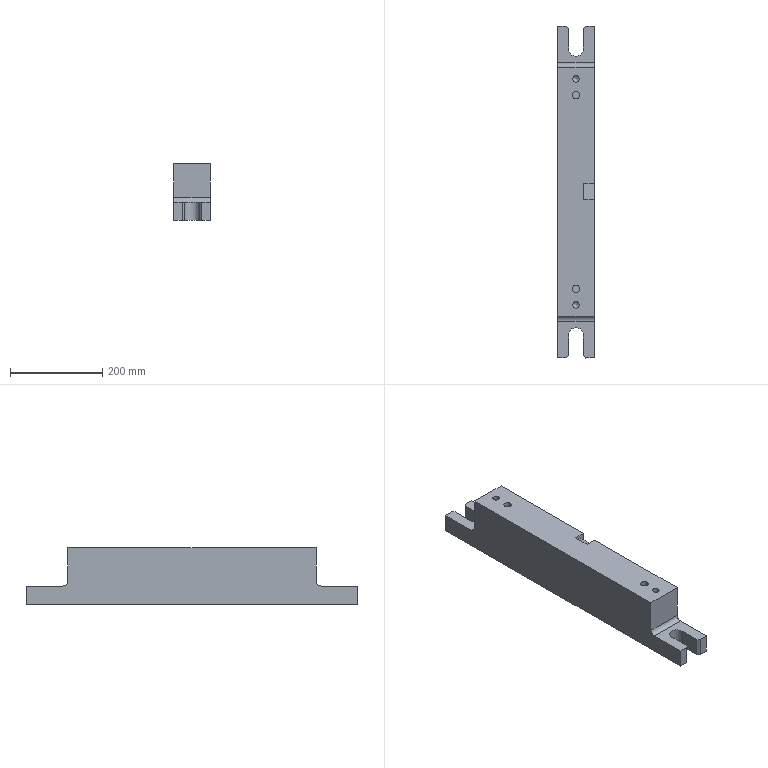Part | NX | features LIN_SOLID_COLOR 2 | 1 solid | 35 faces | box 80 x 720 x 123.5 mm | volume 5716892 mm3 | plane 25 | cylinder 8 | cone 2 | commonest cylinder face diameters 14 x2 16.002 x2 20 x2 32 x2
STEP:
#1=CARTESIAN_POINT('',(-314.,270.,-180.));
#2=VERTEX_POINT('',#1);
#3=CARTESIAN_POINT('',(-234.,270.,-180.));
#4=VERTEX_POINT('',#3);
#5=CARTESIAN_POINT('',(-234.,270.,-180.));
#6=DIRECTION('',(-1.,0.,0.));
#7=VECTOR('',#6,1000.);
#8=LINE('',#5,#7);
#9=EDGE_CURVE('',#2,#4,#8,.F.);
#10=ORIENTED_EDGE('',*,*,#9,.F.);
#11=CARTESIAN_POINT('',(-314.,270.,-106.5));
#12=VERTEX_POINT('',#11);
#13=CARTESIAN_POINT('',(-314.,270.,-101.5));
#14=DIRECTION('',(0.,0.,1.));
#15=VECTOR('',#14,1000.);
#16=LINE('',#13,#15);
#17=EDGE_CURVE('',#2,#12,#16,.T.);
#18=ORIENTED_EDGE('',*,*,#17,.T.);
#19=CARTESIAN_POINT('',(-234.,270.,-106.5));
#20=VERTEX_POINT('',#19);
#21=CARTESIAN_POINT('',(-254.,270.,-106.5));
#22=DIRECTION('',(1.,0.,0.));
#23=VECTOR('',#22,1000.);
#24=LINE('',#21,#23);
#25=EDGE_CURVE('',#12,#20,#24,.T.);
#26=ORIENTED_EDGE('',*,*,#25,.T.);
#27=CARTESIAN_POINT('',(-234.,270.,-101.5));
#28=DIRECTION('',(0.,0.,1.));
#29=VECTOR('',#28,1000.);
#30=LINE('',#27,#29);
#31=EDGE_CURVE('',#4,#20,#30,.T.);
#32=ORIENTED_EDGE('',*,*,#31,.F.);
#33=EDGE_LOOP('',(#10,#18,#26,#32));
#34=FACE_BOUND('',#33,.T.);
#35=CARTESIAN_POINT('',(-254.,270.,-101.5));
#36=DIRECTION('',(0.,-1.,0.));
#37=DIRECTION('',(0.,0.,1.));
#38=AXIS2_PLACEMENT_3D('',#35,#36,#37);
#39=PLANE('',#38);
#40=ADVANCED_FACE('',(#34),#39,.F.);
#41=CARTESIAN_POINT('',(-234.,360.,-230.));
#42=VERTEX_POINT('',#41);
#43=CARTESIAN_POINT('',(-234.,-360.,-230.));
#44=VERTEX_POINT('',#43);
#45=CARTESIAN_POINT('',(-234.,0.,-230.));
#46=DIRECTION('',(0.,-1.,0.));
#47=VECTOR('',#46,1000.);
#48=LINE('',#45,#47);
#49=EDGE_CURVE('',#42,#44,#48,.T.);
#50=ORIENTED_EDGE('',*,*,#49,.T.);
#51=CARTESIAN_POINT('',(-253.,-360.,-230.));
#52=VERTEX_POINT('',#51);
#53=CARTESIAN_POINT('',(436.,-360.,-230.));
#54=DIRECTION('',(1.,0.,0.));
#55=VECTOR('',#54,1000.);
#56=LINE('',#53,#55);
#57=EDGE_CURVE('',#52,#44,#56,.T.);
#58=ORIENTED_EDGE('',*,*,#57,.F.);
#59=CARTESIAN_POINT('',(-258.,-355.,-230.));
#60=VERTEX_POINT('',#59);
#61=CARTESIAN_POINT('',(-126144.583,125531.583,-230.));
#62=DIRECTION('',(-0.7071,0.7071,0.));
#63=VECTOR('',#62,1000.);
#64=LINE('',#61,#63);
#65=EDGE_CURVE('',#52,#60,#64,.T.);
#66=ORIENTED_EDGE('',*,*,#65,.T.);
#67=CARTESIAN_POINT('',(-258.,-310.,-230.));
#68=VERTEX_POINT('',#67);
#69=CARTESIAN_POINT('',(-258.,-1858.277,-230.));
#70=DIRECTION('',(0.,-1.,0.));
#71=VECTOR('',#70,1000.);
#72=LINE('',#69,#71);
#73=EDGE_CURVE('',#68,#60,#72,.T.);
#74=ORIENTED_EDGE('',*,*,#73,.F.);
#75=CARTESIAN_POINT('',(-290.,-310.,-230.));
#76=VERTEX_POINT('',#75);
#77=CARTESIAN_POINT('',(-274.,-310.,-230.));
#78=DIRECTION('',(0.,0.,-1.));
#79=DIRECTION('',(-1.,0.,0.));
#80=AXIS2_PLACEMENT_3D('',#77,#78,#79);
#81=CIRCLE('',#80,16.);
#82=EDGE_CURVE('',#76,#68,#81,.T.);
#83=ORIENTED_EDGE('',*,*,#82,.F.);
#84=CARTESIAN_POINT('',(-290.,-355.,-230.));
#85=VERTEX_POINT('',#84);
#86=CARTESIAN_POINT('',(-290.,-1858.277,-230.));
#87=DIRECTION('',(0.,1.,0.));
#88=VECTOR('',#87,1000.);
#89=LINE('',#86,#88);
#90=EDGE_CURVE('',#85,#76,#89,.T.);
#91=ORIENTED_EDGE('',*,*,#90,.F.);
#92=CARTESIAN_POINT('',(-295.,-360.,-230.));
#93=VERTEX_POINT('',#92);
#94=CARTESIAN_POINT('',(-127663.859,-127728.859,-230.));
#95=DIRECTION('',(-0.7071,-0.7071,0.));
#96=VECTOR('',#95,1000.);
#97=LINE('',#94,#96);
#98=EDGE_CURVE('',#85,#93,#97,.T.);
#99=ORIENTED_EDGE('',*,*,#98,.T.);
#100=CARTESIAN_POINT('',(-314.,-360.,-230.));
#101=VERTEX_POINT('',#100);
#102=CARTESIAN_POINT('',(436.,-360.,-230.));
#103=DIRECTION('',(1.,0.,0.));
#104=VECTOR('',#103,1000.);
#105=LINE('',#102,#104);
#106=EDGE_CURVE('',#101,#93,#105,.T.);
#107=ORIENTED_EDGE('',*,*,#106,.F.);
#108=CARTESIAN_POINT('',(-314.,360.,-230.));
#109=VERTEX_POINT('',#108);
#110=CARTESIAN_POINT('',(-314.,0.,-230.));
#111=DIRECTION('',(0.,-1.,0.));
#112=VECTOR('',#111,1000.);
#113=LINE('',#110,#112);
#114=EDGE_CURVE('',#109,#101,#113,.T.);
#115=ORIENTED_EDGE('',*,*,#114,.F.);
#116=CARTESIAN_POINT('',(-295.,360.,-230.));
#117=VERTEX_POINT('',#116);
#118=CARTESIAN_POINT('',(436.,360.,-230.));
#119=DIRECTION('',(1.,0.,0.));
#120=VECTOR('',#119,1000.);
#121=LINE('',#118,#120);
#122=EDGE_CURVE('',#109,#117,#121,.T.);
#123=ORIENTED_EDGE('',*,*,#122,.T.);
#124=CARTESIAN_POINT('',(-290.,355.,-230.));
#125=VERTEX_POINT('',#124);
#126=CARTESIAN_POINT('',(-127663.859,127728.859,-230.));
#127=DIRECTION('',(-0.7071,0.7071,0.));
#128=VECTOR('',#127,1000.);
#129=LINE('',#126,#128);
#130=EDGE_CURVE('',#125,#117,#129,.T.);
#131=ORIENTED_EDGE('',*,*,#130,.F.);
#132=CARTESIAN_POINT('',(-290.,310.,-230.));
#133=VERTEX_POINT('',#132);
#134=CARTESIAN_POINT('',(-290.,1858.277,-230.));
#135=DIRECTION('',(0.,-1.,0.));
#136=VECTOR('',#135,1000.);
#137=LINE('',#134,#136);
#138=EDGE_CURVE('',#125,#133,#137,.T.);
#139=ORIENTED_EDGE('',*,*,#138,.T.);
#140=CARTESIAN_POINT('',(-258.,310.,-230.));
#141=VERTEX_POINT('',#140);
#142=CARTESIAN_POINT('',(-274.,310.,-230.));
#143=DIRECTION('',(0.,0.,1.));
#144=DIRECTION('',(-1.,0.,0.));
#145=AXIS2_PLACEMENT_3D('',#142,#143,#144);
#146=CIRCLE('',#145,16.);
#147=EDGE_CURVE('',#133,#141,#146,.T.);
#148=ORIENTED_EDGE('',*,*,#147,.T.);
#149=CARTESIAN_POINT('',(-258.,355.,-230.));
#150=VERTEX_POINT('',#149);
#151=CARTESIAN_POINT('',(-258.,1858.277,-230.));
#152=DIRECTION('',(0.,1.,0.));
#153=VECTOR('',#152,1000.);
#154=LINE('',#151,#153);
#155=EDGE_CURVE('',#141,#150,#154,.T.);
#156=ORIENTED_EDGE('',*,*,#155,.T.);
#157=CARTESIAN_POINT('',(-253.,360.,-230.));
#158=VERTEX_POINT('',#157);
#159=CARTESIAN_POINT('',(-126144.583,-125531.583,-230.));
#160=DIRECTION('',(-0.7071,-0.7071,0.));
#161=VECTOR('',#160,1000.);
#162=LINE('',#159,#161);
#163=EDGE_CURVE('',#158,#150,#162,.T.);
#164=ORIENTED_EDGE('',*,*,#163,.F.);
#165=CARTESIAN_POINT('',(436.,360.,-230.));
#166=DIRECTION('',(1.,0.,0.));
#167=VECTOR('',#166,1000.);
#168=LINE('',#165,#167);
#169=EDGE_CURVE('',#158,#42,#168,.T.);
#170=ORIENTED_EDGE('',*,*,#169,.T.);
#171=EDGE_LOOP('',(#50,#58,#66,#74,#83,#91,#99,#107,#115,#123,#131,#139,#148,#156,#164,#170));
#172=FACE_BOUND('',#171,.T.);
#173=CARTESIAN_POINT('',(-114.,0.,-230.));
#174=DIRECTION('',(0.,0.,1.));
#175=DIRECTION('',(1.,0.,0.));
#176=AXIS2_PLACEMENT_3D('',#173,#174,#175);
#177=PLANE('',#176);
#178=ADVANCED_FACE('',(#172),#177,.F.);
#179=CARTESIAN_POINT('',(-234.,-270.,-106.5));
#180=VERTEX_POINT('',#179);
#181=CARTESIAN_POINT('',(-234.,-17.5,-106.5));
#182=VERTEX_POINT('',#181);
#183=CARTESIAN_POINT('',(-234.,0.,-106.5));
#184=DIRECTION('',(0.,1.,0.));
#185=VECTOR('',#184,1000.);
#186=LINE('',#183,#185);
#187=EDGE_CURVE('',#180,#182,#186,.T.);
#188=ORIENTED_EDGE('',*,*,#187,.T.);
#189=CARTESIAN_POINT('',(-257.475,-17.5,-106.5));
#190=VERTEX_POINT('',#189);
#191=CARTESIAN_POINT('',(476.,-17.5,-106.5));
#192=DIRECTION('',(-1.,0.,0.));
#193=VECTOR('',#192,1000.);
#194=LINE('',#191,#193);
#195=EDGE_CURVE('',#182,#190,#194,.T.);
#196=ORIENTED_EDGE('',*,*,#195,.T.);
#197=CARTESIAN_POINT('',(-257.475,17.5,-106.5));
#198=VERTEX_POINT('',#197);
#199=CARTESIAN_POINT('',(-257.475,0.,-106.5));
#200=DIRECTION('',(0.,1.,0.));
#201=VECTOR('',#200,1000.);
#202=LINE('',#199,#201);
#203=EDGE_CURVE('',#198,#190,#202,.F.);
#204=ORIENTED_EDGE('',*,*,#203,.F.);
#205=CARTESIAN_POINT('',(-234.,17.5,-106.5));
#206=VERTEX_POINT('',#205);
#207=CARTESIAN_POINT('',(476.,17.5,-106.5));
#208=DIRECTION('',(1.,0.,0.));
#209=VECTOR('',#208,1000.);
#210=LINE('',#207,#209);
#211=EDGE_CURVE('',#198,#206,#210,.T.);
#212=ORIENTED_EDGE('',*,*,#211,.T.);
#213=CARTESIAN_POINT('',(-234.,0.,-106.5));
#214=DIRECTION('',(0.,1.,0.));
#215=VECTOR('',#214,1000.);
#216=LINE('',#213,#215);
#217=EDGE_CURVE('',#206,#20,#216,.T.);
#218=ORIENTED_EDGE('',*,*,#217,.T.);
#219=ORIENTED_EDGE('',*,*,#25,.F.);
#220=CARTESIAN_POINT('',(-314.,-270.,-106.5));
#221=VERTEX_POINT('',#220);
#222=CARTESIAN_POINT('',(-314.,0.,-106.5));
#223=DIRECTION('',(0.,1.,0.));
#224=VECTOR('',#223,1000.);
#225=LINE('',#222,#224);
#226=EDGE_CURVE('',#221,#12,#225,.T.);
#227=ORIENTED_EDGE('',*,*,#226,.F.);
#228=CARTESIAN_POINT('',(476.,-270.,-106.5));
#229=DIRECTION('',(-1.,0.,0.));
#230=VECTOR('',#229,1000.);
#231=LINE('',#228,#230);
#232=EDGE_CURVE('',#180,#221,#231,.T.);
#233=ORIENTED_EDGE('',*,*,#232,.F.);
#234=EDGE_LOOP('',(#188,#196,#204,#212,#218,#219,#227,#233));
#235=FACE_BOUND('',#234,.T.);
#236=CARTESIAN_POINT('',(-282.001,-210.,-106.5));
#237=VERTEX_POINT('',#236);
#238=CARTESIAN_POINT('',(-274.,-210.,-106.5));
#239=DIRECTION('',(0.,0.,-1.));
#240=DIRECTION('',(-1.,0.,0.));
#241=AXIS2_PLACEMENT_3D('',#238,#239,#240);
#242=CIRCLE('',#241,8.001);
#243=EDGE_CURVE('',#237,#237,#242,.F.);
#244=ORIENTED_EDGE('',*,*,#243,.F.);
#245=EDGE_LOOP('',(#244));
#246=FACE_BOUND('',#245,.T.);
#247=CARTESIAN_POINT('',(-281.,-245.,-106.5));
#248=VERTEX_POINT('',#247);
#249=CARTESIAN_POINT('',(-274.,-245.,-106.5));
#250=DIRECTION('',(0.,0.,-1.));
#251=DIRECTION('',(-1.,0.,0.));
#252=AXIS2_PLACEMENT_3D('',#249,#250,#251);
#253=CIRCLE('',#252,7.);
#254=EDGE_CURVE('',#248,#248,#253,.T.);
#255=ORIENTED_EDGE('',*,*,#254,.T.);
#256=EDGE_LOOP('',(#255));
#257=FACE_BOUND('',#256,.T.);
#258=CARTESIAN_POINT('',(-281.,245.,-106.5));
#259=VERTEX_POINT('',#258);
#260=CARTESIAN_POINT('',(-274.,245.,-106.5));
#261=DIRECTION('',(0.,0.,-1.));
#262=DIRECTION('',(-1.,0.,0.));
#263=AXIS2_PLACEMENT_3D('',#260,#261,#262);
#264=CIRCLE('',#263,7.);
#265=EDGE_CURVE('',#259,#259,#264,.T.);
#266=ORIENTED_EDGE('',*,*,#265,.T.);
#267=EDGE_LOOP('',(#266));
#268=FACE_BOUND('',#267,.T.);
#269=CARTESIAN_POINT('',(-282.001,210.,-106.5));
#270=VERTEX_POINT('',#269);
#271=CARTESIAN_POINT('',(-274.,210.,-106.5));
#272=DIRECTION('',(0.,0.,-1.));
#273=DIRECTION('',(-1.,0.,0.));
#274=AXIS2_PLACEMENT_3D('',#271,#272,#273);
#275=CIRCLE('',#274,8.001);
#276=EDGE_CURVE('',#270,#270,#275,.T.);
#277=ORIENTED_EDGE('',*,*,#276,.T.);
#278=EDGE_LOOP('',(#277));
#279=FACE_BOUND('',#278,.T.);
#280=CARTESIAN_POINT('',(476.,0.,-106.5));
#281=DIRECTION('',(0.,0.,-1.));
#282=DIRECTION('',(-1.,0.,0.));
#283=AXIS2_PLACEMENT_3D('',#280,#281,#282);
#284=PLANE('',#283);
#285=ADVANCED_FACE('',(#235,#246,#257,#268,#279),#284,.F.);
#286=CARTESIAN_POINT('',(-234.,17.5,-122.937));
#287=VERTEX_POINT('',#286);
#288=CARTESIAN_POINT('',(-234.,17.5,-101.5));
#289=DIRECTION('',(0.,0.,-1.));
#290=VECTOR('',#289,1000.);
#291=LINE('',#288,#290);
#292=EDGE_CURVE('',#206,#287,#291,.T.);
#293=ORIENTED_EDGE('',*,*,#292,.T.);
#294=CARTESIAN_POINT('',(-234.,-17.5,-122.937));
#295=VERTEX_POINT('',#294);
#296=CARTESIAN_POINT('',(-234.,0.,-122.937));
#297=DIRECTION('',(0.,-1.,0.));
#298=VECTOR('',#297,1000.);
#299=LINE('',#296,#298);
#300=EDGE_CURVE('',#295,#287,#299,.F.);
#301=ORIENTED_EDGE('',*,*,#300,.F.);
#302=CARTESIAN_POINT('',(-234.,-17.5,-101.5));
#303=DIRECTION('',(0.,0.,1.));
#304=VECTOR('',#303,1000.);
#305=LINE('',#302,#304);
#306=EDGE_CURVE('',#295,#182,#305,.T.);
#307=ORIENTED_EDGE('',*,*,#306,.T.);
#308=ORIENTED_EDGE('',*,*,#187,.F.);
#309=CARTESIAN_POINT('',(-234.,-270.,-180.));
#310=VERTEX_POINT('',#309);
#311=CARTESIAN_POINT('',(-234.,-270.,-101.5));
#312=DIRECTION('',(0.,0.,1.));
#313=VECTOR('',#312,1000.);
#314=LINE('',#311,#313);
#315=EDGE_CURVE('',#310,#180,#314,.T.);
#316=ORIENTED_EDGE('',*,*,#315,.F.);
#317=CARTESIAN_POINT('',(-234.,-280.,-190.));
#318=VERTEX_POINT('',#317);
#319=CARTESIAN_POINT('',(-234.,-280.,-180.));
#320=DIRECTION('',(-1.,0.,0.));
#321=DIRECTION('',(0.,0.,1.));
#322=AXIS2_PLACEMENT_3D('',#319,#320,#321);
#323=CIRCLE('',#322,10.);
#324=EDGE_CURVE('',#310,#318,#323,.T.);
#325=ORIENTED_EDGE('',*,*,#324,.T.);
#326=CARTESIAN_POINT('',(-234.,-360.,-190.));
#327=VERTEX_POINT('',#326);
#328=CARTESIAN_POINT('',(-234.,-320.,-190.));
#329=DIRECTION('',(0.,-1.,0.));
#330=VECTOR('',#329,1000.);
#331=LINE('',#328,#330);
#332=EDGE_CURVE('',#318,#327,#331,.T.);
#333=ORIENTED_EDGE('',*,*,#332,.T.);
#334=CARTESIAN_POINT('',(-234.,-360.,-131.5));
#335=DIRECTION('',(0.,0.,1.));
#336=VECTOR('',#335,1000.);
#337=LINE('',#334,#336);
#338=EDGE_CURVE('',#44,#327,#337,.T.);
#339=ORIENTED_EDGE('',*,*,#338,.F.);
#340=ORIENTED_EDGE('',*,*,#49,.F.);
#341=CARTESIAN_POINT('',(-234.,360.,-190.));
#342=VERTEX_POINT('',#341);
#343=CARTESIAN_POINT('',(-234.,360.,-131.5));
#344=DIRECTION('',(0.,0.,1.));
#345=VECTOR('',#344,1000.);
#346=LINE('',#343,#345);
#347=EDGE_CURVE('',#42,#342,#346,.T.);
#348=ORIENTED_EDGE('',*,*,#347,.T.);
#349=CARTESIAN_POINT('',(-234.,280.,-190.));
#350=VERTEX_POINT('',#349);
#351=CARTESIAN_POINT('',(-234.,320.,-190.));
#352=DIRECTION('',(0.,1.,0.));
#353=VECTOR('',#352,1000.);
#354=LINE('',#351,#353);
#355=EDGE_CURVE('',#350,#342,#354,.T.);
#356=ORIENTED_EDGE('',*,*,#355,.F.);
#357=CARTESIAN_POINT('',(-234.,280.,-180.));
#358=DIRECTION('',(1.,0.,0.));
#359=DIRECTION('',(0.,0.,1.));
#360=AXIS2_PLACEMENT_3D('',#357,#358,#359);
#361=CIRCLE('',#360,10.);
#362=EDGE_CURVE('',#4,#350,#361,.T.);
#363=ORIENTED_EDGE('',*,*,#362,.F.);
#364=ORIENTED_EDGE('',*,*,#31,.T.);
#365=ORIENTED_EDGE('',*,*,#217,.F.);
#366=EDGE_LOOP('',(#293,#301,#307,#308,#316,#325,#333,#339,#340,#348,#356,#363,#364,#365));
#367=FACE_BOUND('',#366,.T.);
#368=CARTESIAN_POINT('',(-234.,0.,-101.5));
#369=DIRECTION('',(-1.,0.,0.));
#370=DIRECTION('',(0.,0.,1.));
#371=AXIS2_PLACEMENT_3D('',#368,#369,#370);
#372=PLANE('',#371);
#373=ADVANCED_FACE('',(#367),#372,.F.);
#374=ORIENTED_EDGE('',*,*,#114,.T.);
#375=CARTESIAN_POINT('',(-314.,-360.,-190.));
#376=VERTEX_POINT('',#375);
#377=CARTESIAN_POINT('',(-314.,-360.,-111.5));
#378=DIRECTION('',(0.,0.,1.));
#379=VECTOR('',#378,1000.);
#380=LINE('',#377,#379);
#381=EDGE_CURVE('',#101,#376,#380,.T.);
#382=ORIENTED_EDGE('',*,*,#381,.T.);
#383=CARTESIAN_POINT('',(-314.,-280.,-190.));
#384=VERTEX_POINT('',#383);
#385=CARTESIAN_POINT('',(-314.,-10.,-190.));
#386=DIRECTION('',(0.,1.,0.));
#387=VECTOR('',#386,1000.);
#388=LINE('',#385,#387);
#389=EDGE_CURVE('',#376,#384,#388,.T.);
#390=ORIENTED_EDGE('',*,*,#389,.T.);
#391=CARTESIAN_POINT('',(-314.,-270.,-180.));
#392=VERTEX_POINT('',#391);
#393=CARTESIAN_POINT('',(-314.,-280.,-180.));
#394=DIRECTION('',(-1.,0.,0.));
#395=DIRECTION('',(0.,0.,1.));
#396=AXIS2_PLACEMENT_3D('',#393,#394,#395);
#397=CIRCLE('',#396,10.);
#398=EDGE_CURVE('',#384,#392,#397,.F.);
#399=ORIENTED_EDGE('',*,*,#398,.T.);
#400=CARTESIAN_POINT('',(-314.,-270.,-101.5));
#401=DIRECTION('',(0.,0.,1.));
#402=VECTOR('',#401,1000.);
#403=LINE('',#400,#402);
#404=EDGE_CURVE('',#221,#392,#403,.F.);
#405=ORIENTED_EDGE('',*,*,#404,.F.);
#406=ORIENTED_EDGE('',*,*,#226,.T.);
#407=ORIENTED_EDGE('',*,*,#17,.F.);
#408=CARTESIAN_POINT('',(-314.,280.,-190.));
#409=VERTEX_POINT('',#408);
#410=CARTESIAN_POINT('',(-314.,280.,-180.));
#411=DIRECTION('',(1.,0.,0.));
#412=DIRECTION('',(0.,0.,1.));
#413=AXIS2_PLACEMENT_3D('',#410,#411,#412);
#414=CIRCLE('',#413,10.);
#415=EDGE_CURVE('',#409,#2,#414,.F.);
#416=ORIENTED_EDGE('',*,*,#415,.F.);
#417=CARTESIAN_POINT('',(-314.,360.,-190.));
#418=VERTEX_POINT('',#417);
#419=CARTESIAN_POINT('',(-314.,10.,-190.));
#420=DIRECTION('',(0.,-1.,0.));
#421=VECTOR('',#420,1000.);
#422=LINE('',#419,#421);
#423=EDGE_CURVE('',#418,#409,#422,.T.);
#424=ORIENTED_EDGE('',*,*,#423,.F.);
#425=CARTESIAN_POINT('',(-314.,360.,-111.5));
#426=DIRECTION('',(0.,0.,1.));
#427=VECTOR('',#426,1000.);
#428=LINE('',#425,#427);
#429=EDGE_CURVE('',#109,#418,#428,.T.);
#430=ORIENTED_EDGE('',*,*,#429,.F.);
#431=EDGE_LOOP('',(#374,#382,#390,#399,#405,#406,#407,#416,#424,#430));
#432=FACE_BOUND('',#431,.T.);
#433=CARTESIAN_POINT('',(-314.,0.,-101.5));
#434=DIRECTION('',(-1.,0.,0.));
#435=DIRECTION('',(0.,0.,1.));
#436=AXIS2_PLACEMENT_3D('',#433,#434,#435);
#437=PLANE('',#436);
#438=ADVANCED_FACE('',(#432),#437,.T.);
#439=CARTESIAN_POINT('',(-267.,-245.,-146.5));
#440=VERTEX_POINT('',#439);
#441=CARTESIAN_POINT('',(-274.,-245.,-146.5));
#442=DIRECTION('',(0.,0.,1.));
#443=DIRECTION('',(1.,0.,0.));
#444=AXIS2_PLACEMENT_3D('',#441,#442,#443);
#445=CIRCLE('',#444,7.);
#446=EDGE_CURVE('',#440,#440,#445,.T.);
#447=ORIENTED_EDGE('',*,*,#446,.F.);
#448=EDGE_LOOP('',(#447));
#449=FACE_BOUND('',#448,.T.);
#450=ORIENTED_EDGE('',*,*,#254,.F.);
#451=EDGE_LOOP('',(#450));
#452=FACE_BOUND('',#451,.T.);
#453=CARTESIAN_POINT('',(-274.,-245.,-106.4));
#454=DIRECTION('',(0.,0.,-1.));
#455=DIRECTION('',(1.,0.,0.));
#456=AXIS2_PLACEMENT_3D('',#453,#454,#455);
#457=CYLINDRICAL_SURFACE('',#456,7.);
#458=ADVANCED_FACE('',(#449,#452),#457,.F.);
#459=ORIENTED_EDGE('',*,*,#446,.T.);
#460=EDGE_LOOP('',(#459));
#461=FACE_BOUND('',#460,.T.);
#462=CARTESIAN_POINT('',(-274.,-245.,-150.541));
#463=VERTEX_POINT('',#462);
#464=VERTEX_LOOP('',#463);
#465=FACE_BOUND('',#464,.T.);
#466=CARTESIAN_POINT('',(-274.,-245.,-150.541));
#467=DIRECTION('',(0.,0.,1.));
#468=DIRECTION('',(1.,0.,0.));
#469=AXIS2_PLACEMENT_3D('',#466,#467,#468);
#470=CONICAL_SURFACE('',#469,0.,1.047);
#471=ADVANCED_FACE('',(#461,#465),#470,.F.);
#472=CARTESIAN_POINT('',(-267.,245.,-146.5));
#473=VERTEX_POINT('',#472);
#474=CARTESIAN_POINT('',(-274.,245.,-146.5));
#475=DIRECTION('',(0.,0.,1.));
#476=DIRECTION('',(1.,0.,0.));
#477=AXIS2_PLACEMENT_3D('',#474,#475,#476);
#478=CIRCLE('',#477,7.);
#479=EDGE_CURVE('',#473,#473,#478,.T.);
#480=ORIENTED_EDGE('',*,*,#479,.F.);
#481=EDGE_LOOP('',(#480));
#482=FACE_BOUND('',#481,.T.);
#483=ORIENTED_EDGE('',*,*,#265,.F.);
#484=EDGE_LOOP('',(#483));
#485=FACE_BOUND('',#484,.T.);
#486=CARTESIAN_POINT('',(-274.,245.,-106.4));
#487=DIRECTION('',(0.,0.,-1.));
#488=DIRECTION('',(1.,0.,0.));
#489=AXIS2_PLACEMENT_3D('',#486,#487,#488);
#490=CYLINDRICAL_SURFACE('',#489,7.);
#491=ADVANCED_FACE('',(#482,#485),#490,.F.);
#492=ORIENTED_EDGE('',*,*,#479,.T.);
#493=EDGE_LOOP('',(#492));
#494=FACE_BOUND('',#493,.T.);
#495=CARTESIAN_POINT('',(-274.,245.,-150.541));
#496=VERTEX_POINT('',#495);
#497=VERTEX_LOOP('',#496);
#498=FACE_BOUND('',#497,.T.);
#499=CARTESIAN_POINT('',(-274.,245.,-150.541));
#500=DIRECTION('',(0.,0.,1.));
#501=DIRECTION('',(1.,0.,0.));
#502=AXIS2_PLACEMENT_3D('',#499,#500,#501);
#503=CONICAL_SURFACE('',#502,0.,1.047);
#504=ADVANCED_FACE('',(#494,#498),#503,.F.);
#505=CARTESIAN_POINT('',(-265.999,210.,-146.5));
#506=VERTEX_POINT('',#505);
#507=CARTESIAN_POINT('',(-274.,210.,-146.5));
#508=DIRECTION('',(0.,0.,1.));
#509=DIRECTION('',(1.,0.,0.));
#510=AXIS2_PLACEMENT_3D('',#507,#508,#509);
#511=CIRCLE('',#510,8.001);
#512=EDGE_CURVE('',#506,#506,#511,.T.);
#513=ORIENTED_EDGE('',*,*,#512,.F.);
#514=EDGE_LOOP('',(#513));
#515=FACE_BOUND('',#514,.T.);
#516=ORIENTED_EDGE('',*,*,#276,.F.);
#517=EDGE_LOOP('',(#516));
#518=FACE_BOUND('',#517,.T.);
#519=CARTESIAN_POINT('',(-274.,210.,-339.5));
#520=DIRECTION('',(0.,0.,1.));
#521=DIRECTION('',(1.,0.,0.));
#522=AXIS2_PLACEMENT_3D('',#519,#520,#521);
#523=CYLINDRICAL_SURFACE('',#522,8.001);
#524=ADVANCED_FACE('',(#515,#518),#523,.F.);
#525=ORIENTED_EDGE('',*,*,#243,.T.);
#526=EDGE_LOOP('',(#525));
#527=FACE_BOUND('',#526,.T.);
#528=CARTESIAN_POINT('',(-265.999,-210.,-146.5));
#529=VERTEX_POINT('',#528);
#530=CARTESIAN_POINT('',(-274.,-210.,-146.5));
#531=DIRECTION('',(0.,0.,1.));
#532=DIRECTION('',(1.,0.,0.));
#533=AXIS2_PLACEMENT_3D('',#530,#531,#532);
#534=CIRCLE('',#533,8.001);
#535=EDGE_CURVE('',#529,#529,#534,.F.);
#536=ORIENTED_EDGE('',*,*,#535,.T.);
#537=EDGE_LOOP('',(#536));
#538=FACE_BOUND('',#537,.T.);
#539=CARTESIAN_POINT('',(-274.,-210.,-304.5));
#540=DIRECTION('',(0.,0.,1.));
#541=DIRECTION('',(1.,0.,0.));
#542=AXIS2_PLACEMENT_3D('',#539,#540,#541);
#543=CYLINDRICAL_SURFACE('',#542,8.001);
#544=ADVANCED_FACE('',(#527,#538),#543,.F.);
#545=ORIENTED_EDGE('',*,*,#404,.T.);
#546=CARTESIAN_POINT('',(-234.,-270.,-180.));
#547=DIRECTION('',(-1.,0.,0.));
#548=VECTOR('',#547,1000.);
#549=LINE('',#546,#548);
#550=EDGE_CURVE('',#392,#310,#549,.F.);
#551=ORIENTED_EDGE('',*,*,#550,.T.);
#552=ORIENTED_EDGE('',*,*,#315,.T.);
#553=ORIENTED_EDGE('',*,*,#232,.T.);
#554=EDGE_LOOP('',(#545,#551,#552,#553));
#555=FACE_BOUND('',#554,.T.);
#556=CARTESIAN_POINT('',(271.,-270.,-71.5));
#557=DIRECTION('',(0.,-1.,0.));
#558=DIRECTION('',(0.,0.,-1.));
#559=AXIS2_PLACEMENT_3D('',#556,#557,#558);
#560=PLANE('',#559);
#561=ADVANCED_FACE('',(#555),#560,.T.);
#562=ORIENTED_EDGE('',*,*,#106,.T.);
#563=CARTESIAN_POINT('',(-295.,-360.,-190.));
#564=VERTEX_POINT('',#563);
#565=CARTESIAN_POINT('',(-295.,-360.,-200.));
#566=DIRECTION('',(0.,0.,1.));
#567=VECTOR('',#566,1000.);
#568=LINE('',#565,#567);
#569=EDGE_CURVE('',#93,#564,#568,.T.);
#570=ORIENTED_EDGE('',*,*,#569,.T.);
#571=CARTESIAN_POINT('',(436.,-360.,-190.));
#572=DIRECTION('',(-1.,0.,0.));
#573=VECTOR('',#572,1000.);
#574=LINE('',#571,#573);
#575=EDGE_CURVE('',#564,#376,#574,.T.);
#576=ORIENTED_EDGE('',*,*,#575,.T.);
#577=ORIENTED_EDGE('',*,*,#381,.F.);
#578=EDGE_LOOP('',(#562,#570,#576,#577));
#579=FACE_BOUND('',#578,.T.);
#580=CARTESIAN_POINT('',(436.,-360.,-131.5));
#581=DIRECTION('',(0.,-1.,0.));
#582=DIRECTION('',(0.,0.,-1.));
#583=AXIS2_PLACEMENT_3D('',#580,#581,#582);
#584=PLANE('',#583);
#585=ADVANCED_FACE('',(#579),#584,.T.);
#586=ORIENTED_EDGE('',*,*,#98,.F.);
#587=CARTESIAN_POINT('',(-290.,-355.,-190.));
#588=VERTEX_POINT('',#587);
#589=CARTESIAN_POINT('',(-290.,-355.,-230.));
#590=DIRECTION('',(0.,0.,-1.));
#591=VECTOR('',#590,1000.);
#592=LINE('',#589,#591);
#593=EDGE_CURVE('',#588,#85,#592,.T.);
#594=ORIENTED_EDGE('',*,*,#593,.F.);
#595=CARTESIAN_POINT('',(-64.5,-129.5,-190.));
#596=DIRECTION('',(0.7071,0.7071,0.));
#597=VECTOR('',#596,1000.);
#598=LINE('',#595,#597);
#599=EDGE_CURVE('',#564,#588,#598,.T.);
#600=ORIENTED_EDGE('',*,*,#599,.F.);
#601=ORIENTED_EDGE('',*,*,#569,.F.);
#602=EDGE_LOOP('',(#586,#594,#600,#601));
#603=FACE_BOUND('',#602,.T.);
#604=CARTESIAN_POINT('',(-295.,-360.,-131.5));
#605=DIRECTION('',(0.7071,-0.7071,0.));
#606=DIRECTION('',(0.,0.,-1.));
#607=AXIS2_PLACEMENT_3D('',#604,#605,#606);
#608=PLANE('',#607);
#609=ADVANCED_FACE('',(#603),#608,.T.);
#610=CARTESIAN_POINT('',(-290.,-310.,-190.));
#611=VERTEX_POINT('',#610);
#612=CARTESIAN_POINT('',(-290.,-30.,-190.));
#613=DIRECTION('',(0.,-1.,0.));
#614=VECTOR('',#613,1000.);
#615=LINE('',#612,#614);
#616=EDGE_CURVE('',#611,#588,#615,.T.);
#617=ORIENTED_EDGE('',*,*,#616,.T.);
#618=ORIENTED_EDGE('',*,*,#593,.T.);
#619=ORIENTED_EDGE('',*,*,#90,.T.);
#620=CARTESIAN_POINT('',(-290.,-310.,-305.));
#621=DIRECTION('',(0.,0.,1.));
#622=VECTOR('',#621,1000.);
#623=LINE('',#620,#622);
#624=EDGE_CURVE('',#611,#76,#623,.F.);
#625=ORIENTED_EDGE('',*,*,#624,.F.);
#626=EDGE_LOOP('',(#617,#618,#619,#625));
#627=FACE_BOUND('',#626,.T.);
#628=CARTESIAN_POINT('',(-290.,-60.,-305.));
#629=DIRECTION('',(-1.,0.,0.));
#630=DIRECTION('',(0.,0.,1.));
#631=AXIS2_PLACEMENT_3D('',#628,#629,#630);
#632=PLANE('',#631);
#633=ADVANCED_FACE('',(#627),#632,.F.);
#634=CARTESIAN_POINT('',(-258.,-310.,-190.));
#635=VERTEX_POINT('',#634);
#636=CARTESIAN_POINT('',(-274.,-310.,-190.));
#637=DIRECTION('',(0.,0.,1.));
#638=DIRECTION('',(1.,0.,0.));
#639=AXIS2_PLACEMENT_3D('',#636,#637,#638);
#640=CIRCLE('',#639,16.);
#641=EDGE_CURVE('',#635,#611,#640,.T.);
#642=ORIENTED_EDGE('',*,*,#641,.T.);
#643=ORIENTED_EDGE('',*,*,#624,.T.);
#644=ORIENTED_EDGE('',*,*,#82,.T.);
#645=CARTESIAN_POINT('',(-258.,-310.,-305.));
#646=DIRECTION('',(0.,0.,-1.));
#647=VECTOR('',#646,1000.);
#648=LINE('',#645,#647);
#649=EDGE_CURVE('',#68,#635,#648,.F.);
#650=ORIENTED_EDGE('',*,*,#649,.T.);
#651=EDGE_LOOP('',(#642,#643,#644,#650));
#652=FACE_BOUND('',#651,.T.);
#653=CARTESIAN_POINT('',(-274.,-310.,-155.));
#654=DIRECTION('',(0.,0.,-1.));
#655=DIRECTION('',(-1.,0.,0.));
#656=AXIS2_PLACEMENT_3D('',#653,#654,#655);
#657=CYLINDRICAL_SURFACE('',#656,16.);
#658=ADVANCED_FACE('',(#652),#657,.F.);
#659=ORIENTED_EDGE('',*,*,#73,.T.);
#660=CARTESIAN_POINT('',(-258.,-355.,-190.));
#661=VERTEX_POINT('',#660);
#662=CARTESIAN_POINT('',(-258.,-355.,-200.));
#663=DIRECTION('',(0.,0.,1.));
#664=VECTOR('',#663,1000.);
#665=LINE('',#662,#664);
#666=EDGE_CURVE('',#60,#661,#665,.T.);
#667=ORIENTED_EDGE('',*,*,#666,.T.);
#668=CARTESIAN_POINT('',(-258.,-30.,-190.));
#669=DIRECTION('',(0.,1.,0.));
#670=VECTOR('',#669,1000.);
#671=LINE('',#668,#670);
#672=EDGE_CURVE('',#661,#635,#671,.T.);
#673=ORIENTED_EDGE('',*,*,#672,.T.);
#674=ORIENTED_EDGE('',*,*,#649,.F.);
#675=EDGE_LOOP('',(#659,#667,#673,#674));
#676=FACE_BOUND('',#675,.T.);
#677=CARTESIAN_POINT('',(-258.,-60.,-305.));
#678=DIRECTION('',(1.,0.,0.));
#679=DIRECTION('',(0.,0.,-1.));
#680=AXIS2_PLACEMENT_3D('',#677,#678,#679);
#681=PLANE('',#680);
#682=ADVANCED_FACE('',(#676),#681,.F.);
#683=ORIENTED_EDGE('',*,*,#65,.F.);
#684=CARTESIAN_POINT('',(-253.,-360.,-190.));
#685=VERTEX_POINT('',#684);
#686=CARTESIAN_POINT('',(-253.,-360.,-230.));
#687=DIRECTION('',(0.,0.,-1.));
#688=VECTOR('',#687,1000.);
#689=LINE('',#686,#688);
#690=EDGE_CURVE('',#685,#52,#689,.T.);
#691=ORIENTED_EDGE('',*,*,#690,.F.);
#692=CARTESIAN_POINT('',(-373.5,-239.5,-190.));
#693=DIRECTION('',(0.7071,-0.7071,0.));
#694=VECTOR('',#693,1000.);
#695=LINE('',#692,#694);
#696=EDGE_CURVE('',#661,#685,#695,.T.);
#697=ORIENTED_EDGE('',*,*,#696,.F.);
#698=ORIENTED_EDGE('',*,*,#666,.F.);
#699=EDGE_LOOP('',(#683,#691,#697,#698));
#700=FACE_BOUND('',#699,.T.);
#701=CARTESIAN_POINT('',(-258.,-355.,-305.));
#702=DIRECTION('',(-0.7071,-0.7071,0.));
#703=DIRECTION('',(0.,0.,-1.));
#704=AXIS2_PLACEMENT_3D('',#701,#702,#703);
#705=PLANE('',#704);
#706=ADVANCED_FACE('',(#700),#705,.T.);
#707=ORIENTED_EDGE('',*,*,#57,.T.);
#708=ORIENTED_EDGE('',*,*,#338,.T.);
#709=CARTESIAN_POINT('',(436.,-360.,-190.));
#710=DIRECTION('',(-1.,0.,0.));
#711=VECTOR('',#710,1000.);
#712=LINE('',#709,#711);
#713=EDGE_CURVE('',#327,#685,#712,.T.);
#714=ORIENTED_EDGE('',*,*,#713,.T.);
#715=ORIENTED_EDGE('',*,*,#690,.T.);
#716=EDGE_LOOP('',(#707,#708,#714,#715));
#717=FACE_BOUND('',#716,.T.);
#718=CARTESIAN_POINT('',(436.,-360.,-131.5));
#719=DIRECTION('',(0.,-1.,0.));
#720=DIRECTION('',(0.,0.,-1.));
#721=AXIS2_PLACEMENT_3D('',#718,#719,#720);
#722=PLANE('',#721);
#723=ADVANCED_FACE('',(#717),#722,.T.);
#724=ORIENTED_EDGE('',*,*,#332,.F.);
#725=CARTESIAN_POINT('',(-314.,-280.,-190.));
#726=DIRECTION('',(-1.,0.,0.));
#727=VECTOR('',#726,1000.);
#728=LINE('',#725,#727);
#729=EDGE_CURVE('',#318,#384,#728,.T.);
#730=ORIENTED_EDGE('',*,*,#729,.T.);
#731=ORIENTED_EDGE('',*,*,#389,.F.);
#732=ORIENTED_EDGE('',*,*,#575,.F.);
#733=ORIENTED_EDGE('',*,*,#599,.T.);
#734=ORIENTED_EDGE('',*,*,#616,.F.);
#735=ORIENTED_EDGE('',*,*,#641,.F.);
#736=ORIENTED_EDGE('',*,*,#672,.F.);
#737=ORIENTED_EDGE('',*,*,#696,.T.);
#738=ORIENTED_EDGE('',*,*,#713,.F.);
#739=EDGE_LOOP('',(#724,#730,#731,#732,#733,#734,#735,#736,#737,#738));
#740=FACE_BOUND('',#739,.T.);
#741=CARTESIAN_POINT('',(-164.,-30.,-190.));
#742=DIRECTION('',(0.,0.,1.));
#743=DIRECTION('',(1.,0.,0.));
#744=AXIS2_PLACEMENT_3D('',#741,#742,#743);
#745=PLANE('',#744);
#746=ADVANCED_FACE('',(#740),#745,.T.);
#747=ORIENTED_EDGE('',*,*,#324,.F.);
#748=ORIENTED_EDGE('',*,*,#550,.F.);
#749=ORIENTED_EDGE('',*,*,#398,.F.);
#750=ORIENTED_EDGE('',*,*,#729,.F.);
#751=EDGE_LOOP('',(#747,#748,#749,#750));
#752=FACE_BOUND('',#751,.T.);
#753=CARTESIAN_POINT('',(-164.,-280.,-180.));
#754=DIRECTION('',(1.,0.,0.));
#755=DIRECTION('',(0.,0.,-1.));
#756=AXIS2_PLACEMENT_3D('',#753,#754,#755);
#757=CYLINDRICAL_SURFACE('',#756,10.);
#758=ADVANCED_FACE('',(#752),#757,.F.);
#759=ORIENTED_EDGE('',*,*,#122,.F.);
#760=ORIENTED_EDGE('',*,*,#429,.T.);
#761=CARTESIAN_POINT('',(-295.,360.,-190.));
#762=VERTEX_POINT('',#761);
#763=CARTESIAN_POINT('',(436.,360.,-190.));
#764=DIRECTION('',(-1.,0.,0.));
#765=VECTOR('',#764,1000.);
#766=LINE('',#763,#765);
#767=EDGE_CURVE('',#762,#418,#766,.T.);
#768=ORIENTED_EDGE('',*,*,#767,.F.);
#769=CARTESIAN_POINT('',(-295.,360.,-200.));
#770=DIRECTION('',(0.,0.,1.));
#771=VECTOR('',#770,1000.);
#772=LINE('',#769,#771);
#773=EDGE_CURVE('',#117,#762,#772,.T.);
#774=ORIENTED_EDGE('',*,*,#773,.F.);
#775=EDGE_LOOP('',(#759,#760,#768,#774));
#776=FACE_BOUND('',#775,.T.);
#777=CARTESIAN_POINT('',(436.,360.,-131.5));
#778=DIRECTION('',(0.,1.,0.));
#779=DIRECTION('',(0.,0.,-1.));
#780=AXIS2_PLACEMENT_3D('',#777,#778,#779);
#781=PLANE('',#780);
#782=ADVANCED_FACE('',(#776),#781,.T.);
#783=ORIENTED_EDGE('',*,*,#130,.T.);
#784=ORIENTED_EDGE('',*,*,#773,.T.);
#785=CARTESIAN_POINT('',(-290.,355.,-190.));
#786=VERTEX_POINT('',#785);
#787=CARTESIAN_POINT('',(-64.5,129.5,-190.));
#788=DIRECTION('',(0.7071,-0.7071,0.));
#789=VECTOR('',#788,1000.);
#790=LINE('',#787,#789);
#791=EDGE_CURVE('',#762,#786,#790,.T.);
#792=ORIENTED_EDGE('',*,*,#791,.T.);
#793=CARTESIAN_POINT('',(-290.,355.,-230.));
#794=DIRECTION('',(0.,0.,-1.));
#795=VECTOR('',#794,1000.);
#796=LINE('',#793,#795);
#797=EDGE_CURVE('',#786,#125,#796,.T.);
#798=ORIENTED_EDGE('',*,*,#797,.T.);
#799=EDGE_LOOP('',(#783,#784,#792,#798));
#800=FACE_BOUND('',#799,.T.);
#801=CARTESIAN_POINT('',(-295.,360.,-131.5));
#802=DIRECTION('',(0.7071,0.7071,0.));
#803=DIRECTION('',(0.,0.,-1.));
#804=AXIS2_PLACEMENT_3D('',#801,#802,#803);
#805=PLANE('',#804);
#806=ADVANCED_FACE('',(#800),#805,.T.);
#807=CARTESIAN_POINT('',(-290.,310.,-190.));
#808=VERTEX_POINT('',#807);
#809=CARTESIAN_POINT('',(-290.,30.,-190.));
#810=DIRECTION('',(0.,1.,0.));
#811=VECTOR('',#810,1000.);
#812=LINE('',#809,#811);
#813=EDGE_CURVE('',#808,#786,#812,.T.);
#814=ORIENTED_EDGE('',*,*,#813,.F.);
#815=CARTESIAN_POINT('',(-290.,310.,-305.));
#816=DIRECTION('',(0.,0.,1.));
#817=VECTOR('',#816,1000.);
#818=LINE('',#815,#817);
#819=EDGE_CURVE('',#808,#133,#818,.F.);
#820=ORIENTED_EDGE('',*,*,#819,.T.);
#821=ORIENTED_EDGE('',*,*,#138,.F.);
#822=ORIENTED_EDGE('',*,*,#797,.F.);
#823=EDGE_LOOP('',(#814,#820,#821,#822));
#824=FACE_BOUND('',#823,.T.);
#825=CARTESIAN_POINT('',(-290.,60.,-305.));
#826=DIRECTION('',(-1.,0.,0.));
#827=DIRECTION('',(0.,0.,1.));
#828=AXIS2_PLACEMENT_3D('',#825,#826,#827);
#829=PLANE('',#828);
#830=ADVANCED_FACE('',(#824),#829,.F.);
#831=CARTESIAN_POINT('',(-258.,310.,-190.));
#832=VERTEX_POINT('',#831);
#833=CARTESIAN_POINT('',(-274.,310.,-190.));
#834=DIRECTION('',(0.,0.,-1.));
#835=DIRECTION('',(1.,0.,0.));
#836=AXIS2_PLACEMENT_3D('',#833,#834,#835);
#837=CIRCLE('',#836,16.);
#838=EDGE_CURVE('',#832,#808,#837,.T.);
#839=ORIENTED_EDGE('',*,*,#838,.F.);
#840=CARTESIAN_POINT('',(-258.,310.,-305.));
#841=DIRECTION('',(0.,0.,-1.));
#842=VECTOR('',#841,1000.);
#843=LINE('',#840,#842);
#844=EDGE_CURVE('',#141,#832,#843,.F.);
#845=ORIENTED_EDGE('',*,*,#844,.F.);
#846=ORIENTED_EDGE('',*,*,#147,.F.);
#847=ORIENTED_EDGE('',*,*,#819,.F.);
#848=EDGE_LOOP('',(#839,#845,#846,#847));
#849=FACE_BOUND('',#848,.T.);
#850=CARTESIAN_POINT('',(-274.,310.,-155.));
#851=DIRECTION('',(0.,0.,-1.));
#852=DIRECTION('',(-1.,0.,0.));
#853=AXIS2_PLACEMENT_3D('',#850,#851,#852);
#854=CYLINDRICAL_SURFACE('',#853,16.);
#855=ADVANCED_FACE('',(#849),#854,.F.);
#856=ORIENTED_EDGE('',*,*,#155,.F.);
#857=ORIENTED_EDGE('',*,*,#844,.T.);
#858=CARTESIAN_POINT('',(-258.,355.,-190.));
#859=VERTEX_POINT('',#858);
#860=CARTESIAN_POINT('',(-258.,30.,-190.));
#861=DIRECTION('',(0.,-1.,0.));
#862=VECTOR('',#861,1000.);
#863=LINE('',#860,#862);
#864=EDGE_CURVE('',#859,#832,#863,.T.);
#865=ORIENTED_EDGE('',*,*,#864,.F.);
#866=CARTESIAN_POINT('',(-258.,355.,-200.));
#867=DIRECTION('',(0.,0.,1.));
#868=VECTOR('',#867,1000.);
#869=LINE('',#866,#868);
#870=EDGE_CURVE('',#150,#859,#869,.T.);
#871=ORIENTED_EDGE('',*,*,#870,.F.);
#872=EDGE_LOOP('',(#856,#857,#865,#871));
#873=FACE_BOUND('',#872,.T.);
#874=CARTESIAN_POINT('',(-258.,60.,-305.));
#875=DIRECTION('',(1.,0.,0.));
#876=DIRECTION('',(0.,0.,-1.));
#877=AXIS2_PLACEMENT_3D('',#874,#875,#876);
#878=PLANE('',#877);
#879=ADVANCED_FACE('',(#873),#878,.F.);
#880=ORIENTED_EDGE('',*,*,#163,.T.);
#881=ORIENTED_EDGE('',*,*,#870,.T.);
#882=CARTESIAN_POINT('',(-253.,360.,-190.));
#883=VERTEX_POINT('',#882);
#884=CARTESIAN_POINT('',(-373.5,239.5,-190.));
#885=DIRECTION('',(0.7071,0.7071,0.));
#886=VECTOR('',#885,1000.);
#887=LINE('',#884,#886);
#888=EDGE_CURVE('',#859,#883,#887,.T.);
#889=ORIENTED_EDGE('',*,*,#888,.T.);
#890=CARTESIAN_POINT('',(-253.,360.,-230.));
#891=DIRECTION('',(0.,0.,-1.));
#892=VECTOR('',#891,1000.);
#893=LINE('',#890,#892);
#894=EDGE_CURVE('',#883,#158,#893,.T.);
#895=ORIENTED_EDGE('',*,*,#894,.T.);
#896=EDGE_LOOP('',(#880,#881,#889,#895));
#897=FACE_BOUND('',#896,.T.);
#898=CARTESIAN_POINT('',(-258.,355.,-305.));
#899=DIRECTION('',(-0.7071,0.7071,0.));
#900=DIRECTION('',(0.,0.,-1.));
#901=AXIS2_PLACEMENT_3D('',#898,#899,#900);
#902=PLANE('',#901);
#903=ADVANCED_FACE('',(#897),#902,.T.);
#904=ORIENTED_EDGE('',*,*,#169,.F.);
#905=ORIENTED_EDGE('',*,*,#894,.F.);
#906=CARTESIAN_POINT('',(436.,360.,-190.));
#907=DIRECTION('',(-1.,0.,0.));
#908=VECTOR('',#907,1000.);
#909=LINE('',#906,#908);
#910=EDGE_CURVE('',#342,#883,#909,.T.);
#911=ORIENTED_EDGE('',*,*,#910,.F.);
#912=ORIENTED_EDGE('',*,*,#347,.F.);
#913=EDGE_LOOP('',(#904,#905,#911,#912));
#914=FACE_BOUND('',#913,.T.);
#915=CARTESIAN_POINT('',(436.,360.,-131.5));
#916=DIRECTION('',(0.,1.,0.));
#917=DIRECTION('',(0.,0.,-1.));
#918=AXIS2_PLACEMENT_3D('',#915,#916,#917);
#919=PLANE('',#918);
#920=ADVANCED_FACE('',(#914),#919,.T.);
#921=ORIENTED_EDGE('',*,*,#355,.T.);
#922=ORIENTED_EDGE('',*,*,#910,.T.);
#923=ORIENTED_EDGE('',*,*,#888,.F.);
#924=ORIENTED_EDGE('',*,*,#864,.T.);
#925=ORIENTED_EDGE('',*,*,#838,.T.);
#926=ORIENTED_EDGE('',*,*,#813,.T.);
#927=ORIENTED_EDGE('',*,*,#791,.F.);
#928=ORIENTED_EDGE('',*,*,#767,.T.);
#929=ORIENTED_EDGE('',*,*,#423,.T.);
#930=CARTESIAN_POINT('',(-314.,280.,-190.));
#931=DIRECTION('',(-1.,0.,0.));
#932=VECTOR('',#931,1000.);
#933=LINE('',#930,#932);
#934=EDGE_CURVE('',#350,#409,#933,.T.);
#935=ORIENTED_EDGE('',*,*,#934,.F.);
#936=EDGE_LOOP('',(#921,#922,#923,#924,#925,#926,#927,#928,#929,#935));
#937=FACE_BOUND('',#936,.T.);
#938=CARTESIAN_POINT('',(-164.,30.,-190.));
#939=DIRECTION('',(0.,0.,1.));
#940=DIRECTION('',(1.,0.,0.));
#941=AXIS2_PLACEMENT_3D('',#938,#939,#940);
#942=PLANE('',#941);
#943=ADVANCED_FACE('',(#937),#942,.T.);
#944=ORIENTED_EDGE('',*,*,#362,.T.);
#945=ORIENTED_EDGE('',*,*,#934,.T.);
#946=ORIENTED_EDGE('',*,*,#415,.T.);
#947=ORIENTED_EDGE('',*,*,#9,.T.);
#948=EDGE_LOOP('',(#944,#945,#946,#947));
#949=FACE_BOUND('',#948,.T.);
#950=CARTESIAN_POINT('',(-164.,280.,-180.));
#951=DIRECTION('',(1.,0.,0.));
#952=DIRECTION('',(0.,0.,-1.));
#953=AXIS2_PLACEMENT_3D('',#950,#951,#952);
#954=CYLINDRICAL_SURFACE('',#953,10.);
#955=ADVANCED_FACE('',(#949),#954,.F.);
#956=ORIENTED_EDGE('',*,*,#306,.F.);
#957=CARTESIAN_POINT('',(-243.07,-17.5,-116.586));
#958=DIRECTION('',(0.8192,0.,-0.5736));
#959=VECTOR('',#958,1000.);
#960=LINE('',#957,#959);
#961=EDGE_CURVE('',#295,#190,#960,.F.);
#962=ORIENTED_EDGE('',*,*,#961,.T.);
#963=ORIENTED_EDGE('',*,*,#195,.F.);
#964=EDGE_LOOP('',(#956,#962,#963));
#965=FACE_BOUND('',#964,.T.);
#966=CARTESIAN_POINT('',(-230.,-17.5,-115.5));
#967=DIRECTION('',(0.,-1.,0.));
#968=DIRECTION('',(0.,0.,-1.));
#969=AXIS2_PLACEMENT_3D('',#966,#967,#968);
#970=PLANE('',#969);
#971=ADVANCED_FACE('',(#965),#970,.F.);
#972=ORIENTED_EDGE('',*,*,#211,.F.);
#973=CARTESIAN_POINT('',(-243.07,17.5,-116.586));
#974=DIRECTION('',(-0.8192,0.,0.5736));
#975=VECTOR('',#974,1000.);
#976=LINE('',#973,#975);
#977=EDGE_CURVE('',#198,#287,#976,.F.);
#978=ORIENTED_EDGE('',*,*,#977,.T.);
#979=ORIENTED_EDGE('',*,*,#292,.F.);
#980=EDGE_LOOP('',(#972,#978,#979));
#981=FACE_BOUND('',#980,.T.);
#982=CARTESIAN_POINT('',(-230.,17.5,-115.5));
#983=DIRECTION('',(0.,1.,0.));
#984=DIRECTION('',(0.,0.,1.));
#985=AXIS2_PLACEMENT_3D('',#982,#983,#984);
#986=PLANE('',#985);
#987=ADVANCED_FACE('',(#981),#986,.F.);
#988=ORIENTED_EDGE('',*,*,#961,.F.);
#989=ORIENTED_EDGE('',*,*,#300,.T.);
#990=ORIENTED_EDGE('',*,*,#977,.F.);
#991=ORIENTED_EDGE('',*,*,#203,.T.);
#992=EDGE_LOOP('',(#988,#989,#990,#991));
#993=FACE_BOUND('',#992,.T.);
#994=CARTESIAN_POINT('',(-243.07,0.,-116.586));
#995=DIRECTION('',(0.5736,0.,0.8192));
#996=DIRECTION('',(0.,-1.,0.));
#997=AXIS2_PLACEMENT_3D('',#994,#995,#996);
#998=PLANE('',#997);
#999=ADVANCED_FACE('',(#993),#998,.T.);
#1000=ORIENTED_EDGE('',*,*,#535,.F.);
#1001=EDGE_LOOP('',(#1000));
#1002=FACE_BOUND('',#1001,.T.);
#1003=CARTESIAN_POINT('',(-274.,-210.,-146.5));
#1004=DIRECTION('',(0.,0.,1.));
#1005=DIRECTION('',(1.,0.,0.));
#1006=AXIS2_PLACEMENT_3D('',#1003,#1004,#1005);
#1007=PLANE('',#1006);
#1008=ADVANCED_FACE('',(#1002),#1007,.T.);
#1009=ORIENTED_EDGE('',*,*,#512,.T.);
#1010=EDGE_LOOP('',(#1009));
#1011=FACE_BOUND('',#1010,.T.);
#1012=CARTESIAN_POINT('',(-274.,210.,-146.5));
#1013=DIRECTION('',(0.,0.,1.));
#1014=DIRECTION('',(1.,0.,0.));
#1015=AXIS2_PLACEMENT_3D('',#1012,#1013,#1014);
#1016=PLANE('',#1015);
#1017=ADVANCED_FACE('',(#1011),#1016,.T.);
#1018=CLOSED_SHELL('',(#40,#178,#285,#373,#438,#458,#471,#491,#504,#524,#544,#561,#585,#609,#633,#658,#682,#706,#723,#746,#758,#782,#806,#830,#855,#879,#903,#920,#943,#955,#971,#987,#999,#1008,#1017));
#1019=MANIFOLD_SOLID_BREP('',#1018);
#1020=(LENGTH_UNIT()NAMED_UNIT(*)SI_UNIT(.MILLI.,.METRE.));
#1021=UNCERTAINTY_MEASURE_WITH_UNIT(LENGTH_MEASURE(0.00001),#1020,'','');
#1022=(NAMED_UNIT(*)PLANE_ANGLE_UNIT()SI_UNIT($,.RADIAN.));
#1023=(NAMED_UNIT(*)SI_UNIT($,.STERADIAN.)SOLID_ANGLE_UNIT());
#1024=(GEOMETRIC_REPRESENTATION_CONTEXT(3)GLOBAL_UNCERTAINTY_ASSIGNED_CONTEXT((#1021))GLOBAL_UNIT_ASSIGNED_CONTEXT((#1020,#1022,#1023))REPRESENTATION_CONTEXT('',''));
#1025=ADVANCED_BREP_SHAPE_REPRESENTATION('',(#1019),#1024);